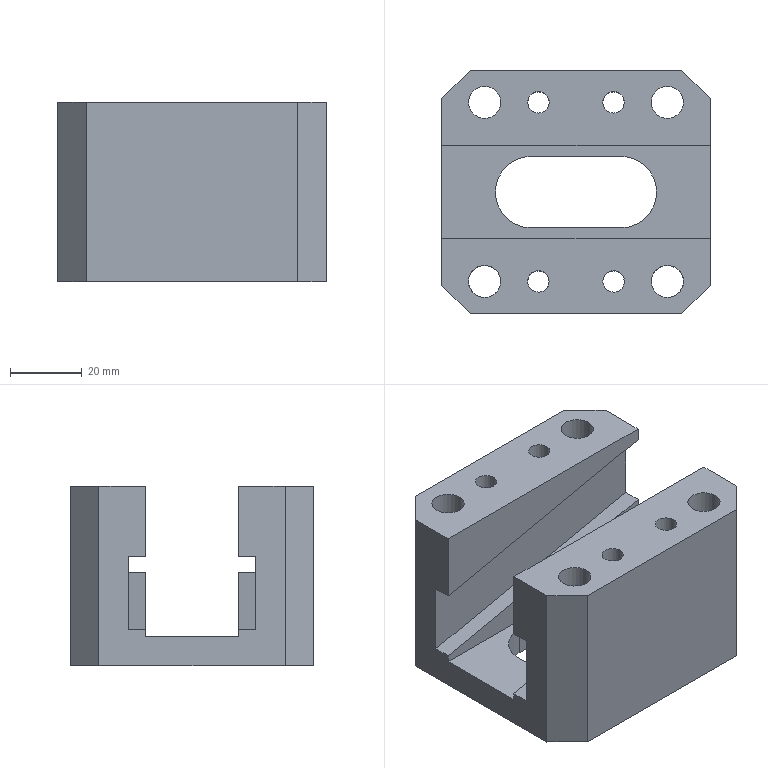Part | STEP file | P011002L002-003 | 1 solid | 42 faces | box 75 x 68 x 50 mm | volume 123835 mm3 | plane 28 | cylinder 14 | commonest cylinder face diameters 6 x4 9 x4 14 x4 20 x2